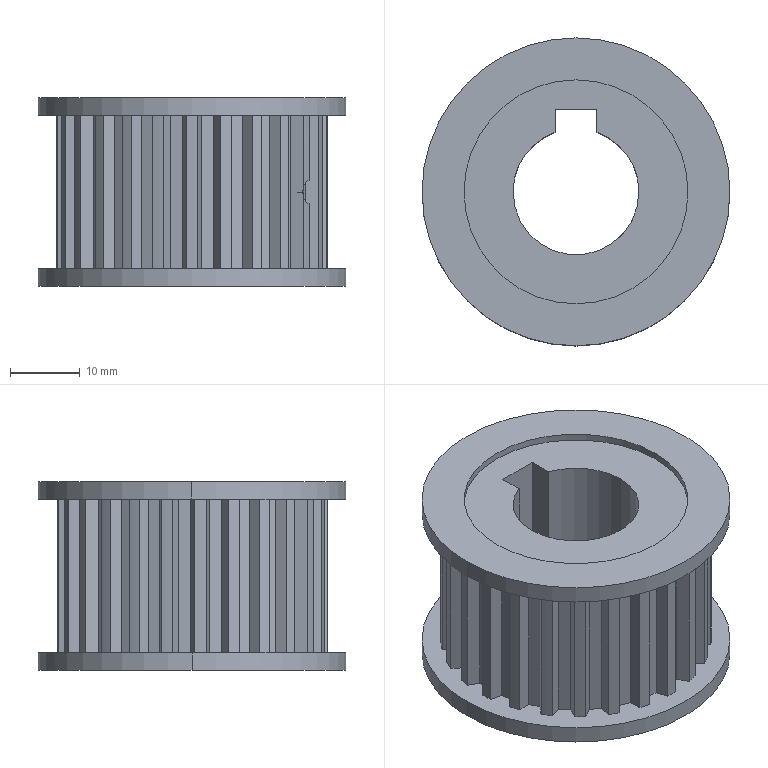Part | SolidWorks | features ICE 4, CirPattern 2, Fillet 2, MirrorPattern 2, Extrusion 1, HoleWzd 1 | 1 solid | 135 faces | box 44 x 44 x 27 mm | volume 22442 mm3 | plane 88 | cylinder 47 | commonest cylinder face diameters 38.65 x26 0.5 x4 3.3 x4 32 x4 44 x4 18 x3